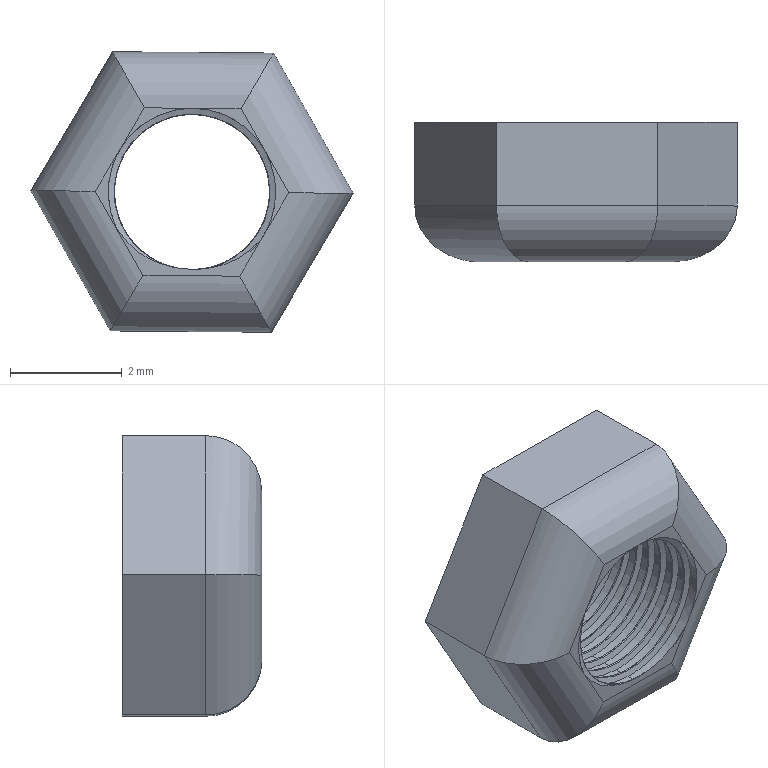Part | SolidWorks | features CombineBodies 1, Extrusion 1, Fillet 1, ICE 1, MoveCopyBody 1, Stock 1 | 1 solid | 39 faces | box 5.773 x 2.5 x 5.023 mm | volume 33.605 mm3 | cylinder 25 | plane 11 | spline 3 | commonest cylinder face diameters 3 x19 2 x6